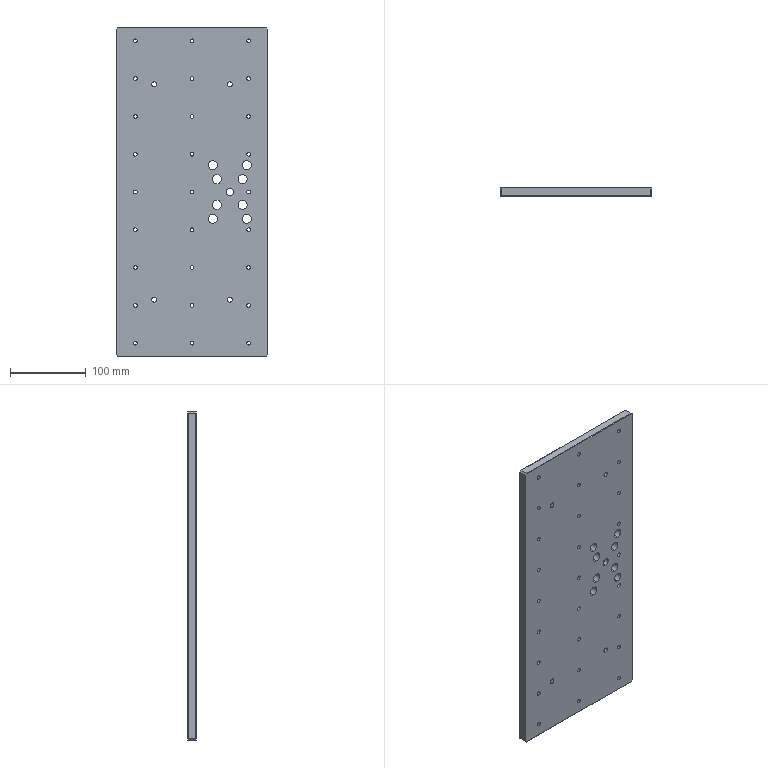Part | STEP file | lift mounting plate | 1 solid | 121 faces | box 200 x 11 x 435 mm | volume 935610 mm3 | cylinder 90 | plane 31 | commonest cylinder face diameters 5 x54 12 x16 6.6 x8 11 x8 10 x2 20 x2